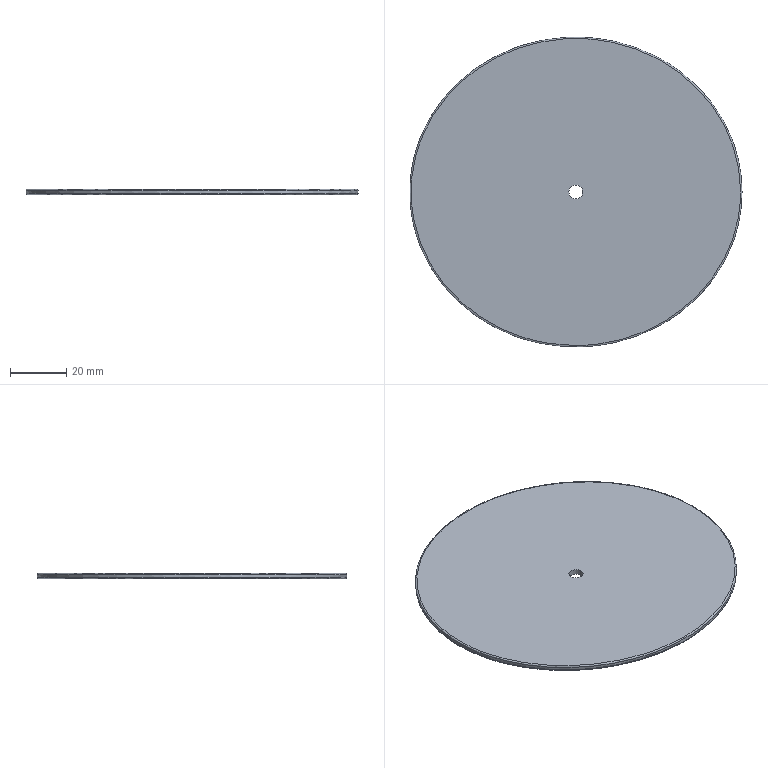Part | NX | features DATUM_CSYS 4, EXTRUDE 3, SKETCH 3, BLEND 1 | 1 solid | 14 faces | box 118.002 x 110 x 2 mm | volume 20001 mm3 | plane 6 | cylinder 5 | spline 3 | commonest cylinder face diameters 10 x4 5 x1